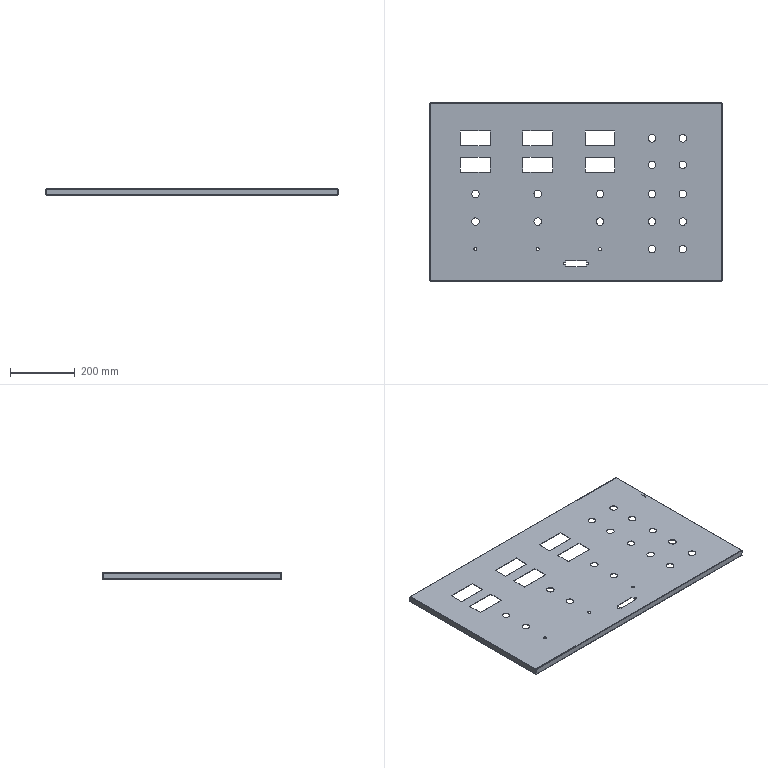Part | SolidWorks | 2 solids | 154 faces | box 900 x 550 x 20 mm | volume 806650 mm3 | plane 79 | cylinder 59 | spline 16 | commonest cylinder face diameters 23 x32 0.2 x8 3.2 x8 9 x6 7 x3 6 x2